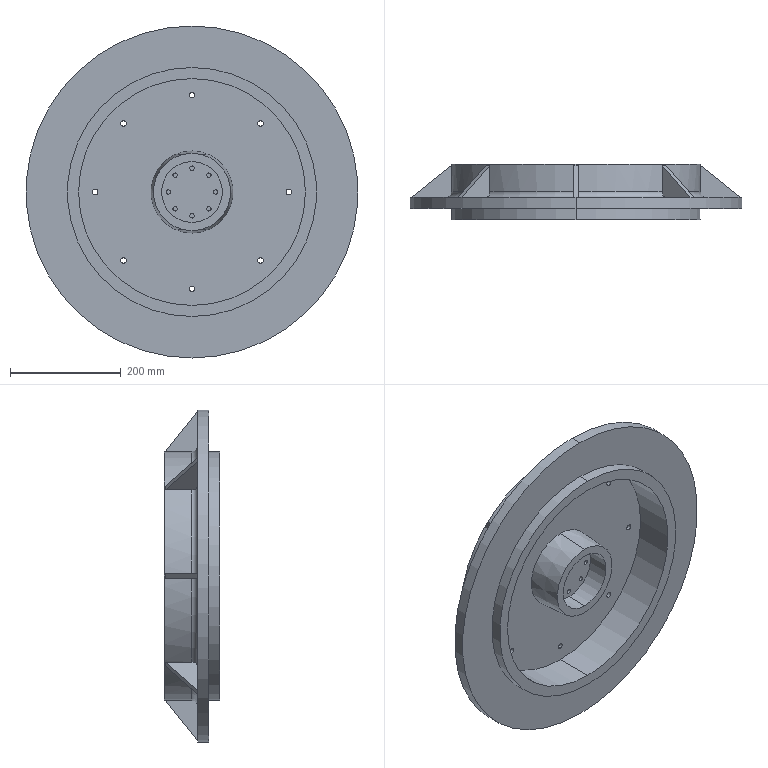Part | SolidWorks | features ICE 10, RefAxis 2, CirPattern 1, MirrorPattern 1, RevCut 1, Revolution 1, Rib 1 | 1 solid | 103 faces | box 600 x 100 x 600 mm | volume 9551199 mm3 | cylinder 46 | plane 43 | torus 8 | cone 6 | commonest cylinder face diameters 8 x16 10 x16 450 x4 110 x2 135 x2 190 x2